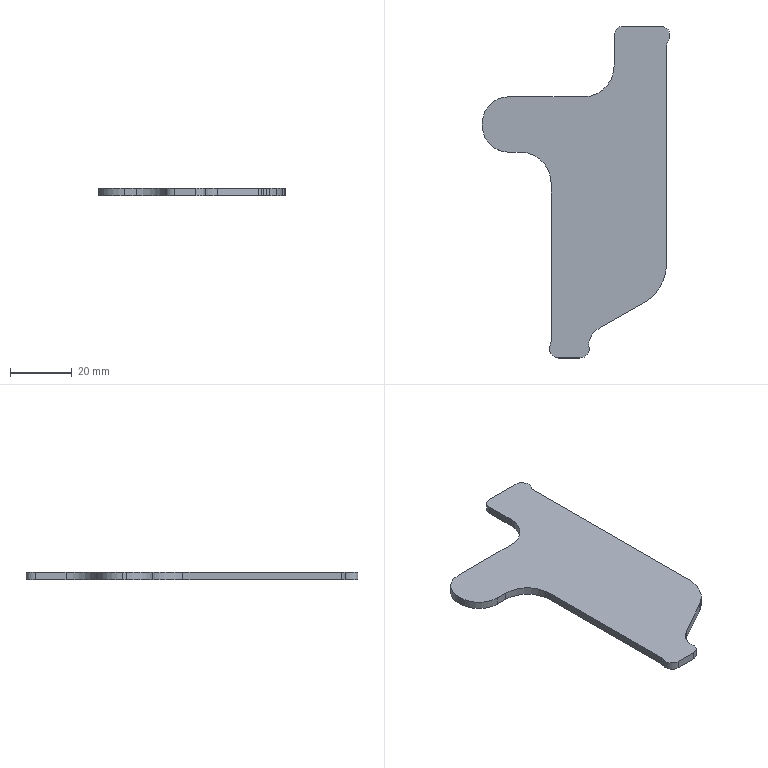Part | STEP file | lll_id354_x_t | 1 solid | 30 faces | box 60.865 x 107.859 x 2.5 mm | volume 9002 mm3 | cylinder 19 | plane 11 | commonest cylinder face diameters 6 x7 17.001 x2 20.001 x2 16.14 x1 25.107 x1 28.276 x1
STEP:
#1=CARTESIAN_POINT('',(469.5,-58.5,0.));
#2=VERTEX_POINT('',#1);
#3=CARTESIAN_POINT('',(469.5,-48.5,0.));
#4=VERTEX_POINT('',#3);
#5=CARTESIAN_POINT('',(469.5,-58.5,0.));
#6=DIRECTION('',(0.,1.,0.));
#7=VECTOR('',#6,1.);
#8=LINE('',#5,#7);
#9=EDGE_CURVE('',#2,#4,#8,.T.);
#10=ORIENTED_EDGE('',*,*,#9,.F.);
#11=CARTESIAN_POINT('',(469.5,-58.5,2.5));
#12=VERTEX_POINT('',#11);
#13=CARTESIAN_POINT('',(469.5,-58.5,2.5));
#14=DIRECTION('',(0.,0.,-1.));
#15=VECTOR('',#14,1.);
#16=LINE('',#13,#15);
#17=EDGE_CURVE('',#12,#2,#16,.T.);
#18=ORIENTED_EDGE('',*,*,#17,.F.);
#19=CARTESIAN_POINT('',(469.5,-48.5,2.5));
#20=VERTEX_POINT('',#19);
#21=CARTESIAN_POINT('',(469.5,-58.5,2.5));
#22=DIRECTION('',(0.,1.,0.));
#23=VECTOR('',#22,1.);
#24=LINE('',#21,#23);
#25=EDGE_CURVE('',#12,#20,#24,.T.);
#26=ORIENTED_EDGE('',*,*,#25,.T.);
#27=CARTESIAN_POINT('',(469.5,-48.5,-2.5));
#28=DIRECTION('',(0.,0.,1.));
#29=VECTOR('',#28,1.);
#30=LINE('',#27,#29);
#31=EDGE_CURVE('',#4,#20,#30,.T.);
#32=ORIENTED_EDGE('',*,*,#31,.F.);
#33=EDGE_LOOP('',(#10,#18,#26,#32));
#34=FACE_OUTER_BOUND('',#33,.T.);
#35=CARTESIAN_POINT('',(469.5,-58.5,2.5));
#36=DIRECTION('',(-1.,0.,0.));
#37=DIRECTION('',(0.,0.,1.));
#38=AXIS2_PLACEMENT_3D('',#35,#36,#37);
#39=PLANE('',#38);
#40=ADVANCED_FACE('',(#34),#39,.T.);
#41=CARTESIAN_POINT('',(459.5,-68.5,0.));
#42=VERTEX_POINT('',#41);
#43=CARTESIAN_POINT('',(459.499,-58.499,0.));
#44=DIRECTION('',(0.,0.,1.));
#45=DIRECTION('',(-1.,0.,0.));
#46=AXIS2_PLACEMENT_3D('',#43,#44,#45);
#47=CIRCLE('',#46,10.001);
#48=EDGE_CURVE('',#42,#2,#47,.T.);
#49=ORIENTED_EDGE('',*,*,#48,.F.);
#50=CARTESIAN_POINT('',(459.5,-68.5,2.5));
#51=VERTEX_POINT('',#50);
#52=CARTESIAN_POINT('',(459.5,-68.5,2.5));
#53=DIRECTION('',(0.,0.,-1.));
#54=VECTOR('',#53,1.);
#55=LINE('',#52,#54);
#56=EDGE_CURVE('',#51,#42,#55,.T.);
#57=ORIENTED_EDGE('',*,*,#56,.F.);
#58=CARTESIAN_POINT('',(459.499,-58.499,2.5));
#59=DIRECTION('',(0.,0.,1.));
#60=DIRECTION('',(-1.,0.,0.));
#61=AXIS2_PLACEMENT_3D('',#58,#59,#60);
#62=CIRCLE('',#61,10.001);
#63=EDGE_CURVE('',#51,#12,#62,.T.);
#64=ORIENTED_EDGE('',*,*,#63,.T.);
#65=ORIENTED_EDGE('',*,*,#17,.T.);
#66=EDGE_LOOP('',(#49,#57,#64,#65));
#67=FACE_OUTER_BOUND('',#66,.T.);
#68=CARTESIAN_POINT('',(459.499,-58.499,2.5));
#69=DIRECTION('',(0.,0.,-1.));
#70=DIRECTION('',(-1.,0.,0.));
#71=AXIS2_PLACEMENT_3D('',#68,#69,#70);
#72=CYLINDRICAL_SURFACE('',#71,10.001);
#73=ADVANCED_FACE('',(#67),#72,.F.);
#74=CARTESIAN_POINT('',(435.2,-68.5,0.));
#75=VERTEX_POINT('',#74);
#76=CARTESIAN_POINT('',(435.2,-68.5,0.));
#77=DIRECTION('',(1.,0.,0.));
#78=VECTOR('',#77,1.);
#79=LINE('',#76,#78);
#80=EDGE_CURVE('',#75,#42,#79,.T.);
#81=ORIENTED_EDGE('',*,*,#80,.F.);
#82=CARTESIAN_POINT('',(435.2,-68.5,2.5));
#83=VERTEX_POINT('',#82);
#84=CARTESIAN_POINT('',(435.2,-68.5,2.5));
#85=DIRECTION('',(0.,0.,-1.));
#86=VECTOR('',#85,1.);
#87=LINE('',#84,#86);
#88=EDGE_CURVE('',#83,#75,#87,.T.);
#89=ORIENTED_EDGE('',*,*,#88,.F.);
#90=CARTESIAN_POINT('',(435.2,-68.5,2.5));
#91=DIRECTION('',(1.,0.,0.));
#92=VECTOR('',#91,1.);
#93=LINE('',#90,#92);
#94=EDGE_CURVE('',#83,#51,#93,.T.);
#95=ORIENTED_EDGE('',*,*,#94,.T.);
#96=ORIENTED_EDGE('',*,*,#56,.T.);
#97=EDGE_LOOP('',(#81,#89,#95,#96));
#98=FACE_OUTER_BOUND('',#97,.T.);
#99=CARTESIAN_POINT('',(435.2,-68.5,2.5));
#100=DIRECTION('',(0.,1.,0.));
#101=DIRECTION('',(0.,0.,1.));
#102=AXIS2_PLACEMENT_3D('',#99,#100,#101);
#103=PLANE('',#102);
#104=ADVANCED_FACE('',(#98),#103,.T.);
#105=CARTESIAN_POINT('',(426.7,-77.,0.));
#106=VERTEX_POINT('',#105);
#107=CARTESIAN_POINT('',(435.2,-77.,0.));
#108=DIRECTION('',(0.,0.,-1.));
#109=DIRECTION('',(-1.,0.,0.));
#110=AXIS2_PLACEMENT_3D('',#107,#108,#109);
#111=CIRCLE('',#110,8.5);
#112=EDGE_CURVE('',#106,#75,#111,.T.);
#113=ORIENTED_EDGE('',*,*,#112,.F.);
#114=CARTESIAN_POINT('',(426.7,-77.,2.5));
#115=VERTEX_POINT('',#114);
#116=CARTESIAN_POINT('',(426.7,-77.,2.5));
#117=DIRECTION('',(0.,0.,-1.));
#118=VECTOR('',#117,1.);
#119=LINE('',#116,#118);
#120=EDGE_CURVE('',#115,#106,#119,.T.);
#121=ORIENTED_EDGE('',*,*,#120,.F.);
#122=CARTESIAN_POINT('',(435.2,-77.,2.5));
#123=DIRECTION('',(0.,0.,-1.));
#124=DIRECTION('',(-1.,0.,0.));
#125=AXIS2_PLACEMENT_3D('',#122,#123,#124);
#126=CIRCLE('',#125,8.5);
#127=EDGE_CURVE('',#115,#83,#126,.T.);
#128=ORIENTED_EDGE('',*,*,#127,.T.);
#129=ORIENTED_EDGE('',*,*,#88,.T.);
#130=EDGE_LOOP('',(#113,#121,#128,#129));
#131=FACE_OUTER_BOUND('',#130,.T.);
#132=CARTESIAN_POINT('',(435.2,-77.,2.5));
#133=DIRECTION('',(0.,0.,-1.));
#134=DIRECTION('',(-1.,0.,0.));
#135=AXIS2_PLACEMENT_3D('',#132,#133,#134);
#136=CYLINDRICAL_SURFACE('',#135,8.5);
#137=ADVANCED_FACE('',(#131),#136,.T.);
#138=CARTESIAN_POINT('',(426.7,-78.,0.));
#139=VERTEX_POINT('',#138);
#140=CARTESIAN_POINT('',(426.7,-78.,0.));
#141=DIRECTION('',(0.,1.,0.));
#142=VECTOR('',#141,1.);
#143=LINE('',#140,#142);
#144=EDGE_CURVE('',#139,#106,#143,.T.);
#145=ORIENTED_EDGE('',*,*,#144,.F.);
#146=CARTESIAN_POINT('',(426.7,-78.,2.5));
#147=VERTEX_POINT('',#146);
#148=CARTESIAN_POINT('',(426.7,-78.,2.5));
#149=DIRECTION('',(0.,0.,-1.));
#150=VECTOR('',#149,1.);
#151=LINE('',#148,#150);
#152=EDGE_CURVE('',#147,#139,#151,.T.);
#153=ORIENTED_EDGE('',*,*,#152,.F.);
#154=CARTESIAN_POINT('',(426.7,-78.,2.5));
#155=DIRECTION('',(0.,1.,0.));
#156=VECTOR('',#155,1.);
#157=LINE('',#154,#156);
#158=EDGE_CURVE('',#147,#115,#157,.T.);
#159=ORIENTED_EDGE('',*,*,#158,.T.);
#160=ORIENTED_EDGE('',*,*,#120,.T.);
#161=EDGE_LOOP('',(#145,#153,#159,#160));
#162=FACE_OUTER_BOUND('',#161,.T.);
#163=CARTESIAN_POINT('',(426.7,-78.,2.5));
#164=DIRECTION('',(-1.,0.,0.));
#165=DIRECTION('',(0.,0.,1.));
#166=AXIS2_PLACEMENT_3D('',#163,#164,#165);
#167=PLANE('',#166);
#168=ADVANCED_FACE('',(#162),#167,.T.);
#169=CARTESIAN_POINT('',(435.2,-86.5,0.));
#170=VERTEX_POINT('',#169);
#171=CARTESIAN_POINT('',(435.2,-78.,0.));
#172=DIRECTION('',(0.,0.,-1.));
#173=DIRECTION('',(-1.,0.,0.));
#174=AXIS2_PLACEMENT_3D('',#171,#172,#173);
#175=CIRCLE('',#174,8.5);
#176=EDGE_CURVE('',#170,#139,#175,.T.);
#177=ORIENTED_EDGE('',*,*,#176,.F.);
#178=CARTESIAN_POINT('',(435.2,-86.5,2.5));
#179=VERTEX_POINT('',#178);
#180=CARTESIAN_POINT('',(435.2,-86.5,2.5));
#181=DIRECTION('',(0.,0.,-1.));
#182=VECTOR('',#181,1.);
#183=LINE('',#180,#182);
#184=EDGE_CURVE('',#179,#170,#183,.T.);
#185=ORIENTED_EDGE('',*,*,#184,.F.);
#186=CARTESIAN_POINT('',(435.2,-78.,2.5));
#187=DIRECTION('',(0.,0.,-1.));
#188=DIRECTION('',(-1.,0.,0.));
#189=AXIS2_PLACEMENT_3D('',#186,#187,#188);
#190=CIRCLE('',#189,8.5);
#191=EDGE_CURVE('',#179,#147,#190,.T.);
#192=ORIENTED_EDGE('',*,*,#191,.T.);
#193=ORIENTED_EDGE('',*,*,#152,.T.);
#194=EDGE_LOOP('',(#177,#185,#192,#193));
#195=FACE_OUTER_BOUND('',#194,.T.);
#196=CARTESIAN_POINT('',(435.2,-78.,2.5));
#197=DIRECTION('',(0.,0.,-1.));
#198=DIRECTION('',(-1.,0.,0.));
#199=AXIS2_PLACEMENT_3D('',#196,#197,#198);
#200=CYLINDRICAL_SURFACE('',#199,8.5);
#201=ADVANCED_FACE('',(#195),#200,.T.);
#202=CARTESIAN_POINT('',(439.,-86.5,0.));
#203=VERTEX_POINT('',#202);
#204=CARTESIAN_POINT('',(439.,-86.5,0.));
#205=DIRECTION('',(-1.,0.,0.));
#206=VECTOR('',#205,1.);
#207=LINE('',#204,#206);
#208=EDGE_CURVE('',#203,#170,#207,.T.);
#209=ORIENTED_EDGE('',*,*,#208,.F.);
#210=CARTESIAN_POINT('',(439.,-86.5,2.5));
#211=VERTEX_POINT('',#210);
#212=CARTESIAN_POINT('',(439.,-86.5,2.5));
#213=DIRECTION('',(0.,0.,-1.));
#214=VECTOR('',#213,1.);
#215=LINE('',#212,#214);
#216=EDGE_CURVE('',#211,#203,#215,.T.);
#217=ORIENTED_EDGE('',*,*,#216,.F.);
#218=CARTESIAN_POINT('',(439.,-86.5,2.5));
#219=DIRECTION('',(-1.,0.,0.));
#220=VECTOR('',#219,1.);
#221=LINE('',#218,#220);
#222=EDGE_CURVE('',#211,#179,#221,.T.);
#223=ORIENTED_EDGE('',*,*,#222,.T.);
#224=ORIENTED_EDGE('',*,*,#184,.T.);
#225=EDGE_LOOP('',(#209,#217,#223,#224));
#226=FACE_OUTER_BOUND('',#225,.T.);
#227=CARTESIAN_POINT('',(439.,-86.5,2.5));
#228=DIRECTION('',(0.,-1.,0.));
#229=DIRECTION('',(0.,0.,-1.));
#230=AXIS2_PLACEMENT_3D('',#227,#228,#229);
#231=PLANE('',#230);
#232=ADVANCED_FACE('',(#226),#231,.T.);
#233=CARTESIAN_POINT('',(449.,-96.5,0.));
#234=VERTEX_POINT('',#233);
#235=CARTESIAN_POINT('',(438.999,-96.501,0.));
#236=DIRECTION('',(0.,0.,1.));
#237=DIRECTION('',(-1.,0.,0.));
#238=AXIS2_PLACEMENT_3D('',#235,#236,#237);
#239=CIRCLE('',#238,10.001);
#240=EDGE_CURVE('',#234,#203,#239,.T.);
#241=ORIENTED_EDGE('',*,*,#240,.F.);
#242=CARTESIAN_POINT('',(449.,-96.5,2.5));
#243=VERTEX_POINT('',#242);
#244=CARTESIAN_POINT('',(449.,-96.5,2.5));
#245=DIRECTION('',(0.,0.,-1.));
#246=VECTOR('',#245,1.);
#247=LINE('',#244,#246);
#248=EDGE_CURVE('',#243,#234,#247,.T.);
#249=ORIENTED_EDGE('',*,*,#248,.F.);
#250=CARTESIAN_POINT('',(438.999,-96.501,2.5));
#251=DIRECTION('',(0.,0.,1.));
#252=DIRECTION('',(-1.,0.,0.));
#253=AXIS2_PLACEMENT_3D('',#250,#251,#252);
#254=CIRCLE('',#253,10.001);
#255=EDGE_CURVE('',#243,#211,#254,.T.);
#256=ORIENTED_EDGE('',*,*,#255,.T.);
#257=ORIENTED_EDGE('',*,*,#216,.T.);
#258=EDGE_LOOP('',(#241,#249,#256,#257));
#259=FACE_OUTER_BOUND('',#258,.T.);
#260=CARTESIAN_POINT('',(438.999,-96.501,2.5));
#261=DIRECTION('',(0.,0.,-1.));
#262=DIRECTION('',(-1.,0.,0.));
#263=AXIS2_PLACEMENT_3D('',#260,#261,#262);
#264=CYLINDRICAL_SURFACE('',#263,10.001);
#265=ADVANCED_FACE('',(#259),#264,.F.);
#266=CARTESIAN_POINT('',(449.,-147.961,0.));
#267=VERTEX_POINT('',#266);
#268=CARTESIAN_POINT('',(449.,-147.961,0.));
#269=DIRECTION('',(0.,1.,0.));
#270=VECTOR('',#269,1.);
#271=LINE('',#268,#270);
#272=EDGE_CURVE('',#267,#234,#271,.T.);
#273=ORIENTED_EDGE('',*,*,#272,.F.);
#274=CARTESIAN_POINT('',(449.,-147.961,2.5));
#275=VERTEX_POINT('',#274);
#276=CARTESIAN_POINT('',(449.,-147.961,2.5));
#277=DIRECTION('',(0.,0.,-1.));
#278=VECTOR('',#277,1.);
#279=LINE('',#276,#278);
#280=EDGE_CURVE('',#275,#267,#279,.T.);
#281=ORIENTED_EDGE('',*,*,#280,.F.);
#282=CARTESIAN_POINT('',(449.,-147.961,2.5));
#283=DIRECTION('',(0.,1.,0.));
#284=VECTOR('',#283,1.);
#285=LINE('',#282,#284);
#286=EDGE_CURVE('',#275,#243,#285,.T.);
#287=ORIENTED_EDGE('',*,*,#286,.T.);
#288=ORIENTED_EDGE('',*,*,#248,.T.);
#289=EDGE_LOOP('',(#273,#281,#287,#288));
#290=FACE_OUTER_BOUND('',#289,.T.);
#291=CARTESIAN_POINT('',(449.,-147.961,2.5));
#292=DIRECTION('',(-1.,0.,0.));
#293=DIRECTION('',(0.,0.,1.));
#294=AXIS2_PLACEMENT_3D('',#291,#292,#293);
#295=PLANE('',#294);
#296=ADVANCED_FACE('',(#290),#295,.T.);
#297=CARTESIAN_POINT('',(448.75,-149.16,0.));
#298=VERTEX_POINT('',#297);
#299=CARTESIAN_POINT('',(446.,-147.961,0.));
#300=DIRECTION('',(0.,0.,1.));
#301=DIRECTION('',(-1.,0.,0.));
#302=AXIS2_PLACEMENT_3D('',#299,#300,#301);
#303=CIRCLE('',#302,3.);
#304=EDGE_CURVE('',#298,#267,#303,.T.);
#305=ORIENTED_EDGE('',*,*,#304,.F.);
#306=CARTESIAN_POINT('',(448.75,-149.16,2.5));
#307=VERTEX_POINT('',#306);
#308=CARTESIAN_POINT('',(448.75,-149.16,2.5));
#309=DIRECTION('',(0.,0.,-1.));
#310=VECTOR('',#309,1.);
#311=LINE('',#308,#310);
#312=EDGE_CURVE('',#307,#298,#311,.T.);
#313=ORIENTED_EDGE('',*,*,#312,.F.);
#314=CARTESIAN_POINT('',(446.,-147.961,2.5));
#315=DIRECTION('',(0.,0.,1.));
#316=DIRECTION('',(-1.,0.,0.));
#317=AXIS2_PLACEMENT_3D('',#314,#315,#316);
#318=CIRCLE('',#317,3.);
#319=EDGE_CURVE('',#307,#275,#318,.T.);
#320=ORIENTED_EDGE('',*,*,#319,.T.);
#321=ORIENTED_EDGE('',*,*,#280,.T.);
#322=EDGE_LOOP('',(#305,#313,#320,#321));
#323=FACE_OUTER_BOUND('',#322,.T.);
#324=CARTESIAN_POINT('',(446.,-147.961,2.5));
#325=DIRECTION('',(0.,0.,-1.));
#326=DIRECTION('',(-1.,0.,0.));
#327=AXIS2_PLACEMENT_3D('',#324,#325,#326);
#328=CYLINDRICAL_SURFACE('',#327,3.);
#329=ADVANCED_FACE('',(#323),#328,.F.);
#330=CARTESIAN_POINT('',(451.5,-153.359,0.));
#331=VERTEX_POINT('',#330);
#332=CARTESIAN_POINT('',(451.5,-150.359,0.));
#333=DIRECTION('',(0.,0.,-1.));
#334=DIRECTION('',(-1.,0.,0.));
#335=AXIS2_PLACEMENT_3D('',#332,#333,#334);
#336=CIRCLE('',#335,3.);
#337=EDGE_CURVE('',#331,#298,#336,.T.);
#338=ORIENTED_EDGE('',*,*,#337,.F.);
#339=CARTESIAN_POINT('',(451.5,-153.359,2.5));
#340=VERTEX_POINT('',#339);
#341=CARTESIAN_POINT('',(451.5,-153.359,2.5));
#342=DIRECTION('',(0.,0.,-1.));
#343=VECTOR('',#342,1.);
#344=LINE('',#341,#343);
#345=EDGE_CURVE('',#340,#331,#344,.T.);
#346=ORIENTED_EDGE('',*,*,#345,.F.);
#347=CARTESIAN_POINT('',(451.5,-150.359,2.5));
#348=DIRECTION('',(0.,0.,-1.));
#349=DIRECTION('',(-1.,0.,0.));
#350=AXIS2_PLACEMENT_3D('',#347,#348,#349);
#351=CIRCLE('',#350,3.);
#352=EDGE_CURVE('',#340,#307,#351,.T.);
#353=ORIENTED_EDGE('',*,*,#352,.T.);
#354=ORIENTED_EDGE('',*,*,#312,.T.);
#355=EDGE_LOOP('',(#338,#346,#353,#354));
#356=FACE_OUTER_BOUND('',#355,.T.);
#357=CARTESIAN_POINT('',(451.5,-150.359,2.5));
#358=DIRECTION('',(0.,0.,-1.));
#359=DIRECTION('',(-1.,0.,0.));
#360=AXIS2_PLACEMENT_3D('',#357,#358,#359);
#361=CYLINDRICAL_SURFACE('',#360,3.);
#362=ADVANCED_FACE('',(#356),#361,.T.);
#363=ORIENTED_EDGE('',*,*,#9,.T.);
#364=CARTESIAN_POINT('',(472.5,-45.5,0.));
#365=VERTEX_POINT('',#364);
#366=CARTESIAN_POINT('',(472.5,-48.5,0.));
#367=DIRECTION('',(0.,0.,-1.));
#368=DIRECTION('',(1.,0.,0.));
#369=AXIS2_PLACEMENT_3D('',#366,#367,#368);
#370=CIRCLE('',#369,3.);
#371=EDGE_CURVE('',#4,#365,#370,.T.);
#372=ORIENTED_EDGE('',*,*,#371,.T.);
#373=CARTESIAN_POINT('',(484.565,-45.5,0.));
#374=VERTEX_POINT('',#373);
#375=CARTESIAN_POINT('',(471.445,-45.5,0.));
#376=DIRECTION('',(1.,0.,0.));
#377=VECTOR('',#376,1.);
#378=LINE('',#375,#377);
#379=EDGE_CURVE('',#365,#374,#378,.T.);
#380=ORIENTED_EDGE('',*,*,#379,.T.);
#381=CARTESIAN_POINT('',(487.038,-50.199,0.));
#382=VERTEX_POINT('',#381);
#383=CARTESIAN_POINT('',(484.565,-48.5,0.));
#384=DIRECTION('',(0.,0.,-1.));
#385=DIRECTION('',(1.,0.,0.));
#386=AXIS2_PLACEMENT_3D('',#383,#384,#385);
#387=CIRCLE('',#386,3.);
#388=EDGE_CURVE('',#374,#382,#387,.T.);
#389=ORIENTED_EDGE('',*,*,#388,.T.);
#390=CARTESIAN_POINT('',(486.51,-51.898,0.));
#391=VERTEX_POINT('',#390);
#392=CARTESIAN_POINT('',(489.51,-51.898,0.));
#393=DIRECTION('',(0.,0.,-1.));
#394=DIRECTION('',(1.,0.,0.));
#395=AXIS2_PLACEMENT_3D('',#392,#393,#394);
#396=CIRCLE('',#395,3.);
#397=EDGE_CURVE('',#391,#382,#396,.T.);
#398=ORIENTED_EDGE('',*,*,#397,.F.);
#399=CARTESIAN_POINT('',(486.506,-122.731,0.));
#400=VERTEX_POINT('',#399);
#401=CARTESIAN_POINT('',(486.51,-51.898,0.));
#402=DIRECTION('',(0.00006142,1.,0.));
#403=VECTOR('',#402,1.);
#404=LINE('',#401,#403);
#405=EDGE_CURVE('',#400,#391,#404,.T.);
#406=ORIENTED_EDGE('',*,*,#405,.F.);
#407=CARTESIAN_POINT('',(486.461,-123.716,0.));
#408=VERTEX_POINT('',#407);
#409=CARTESIAN_POINT('',(439.156,-121.059,0.));
#410=DIRECTION('',(0.,0.,1.));
#411=DIRECTION('',(1.,0.,0.));
#412=AXIS2_PLACEMENT_3D('',#409,#410,#411);
#413=CIRCLE('',#412,47.38);
#414=EDGE_CURVE('',#408,#400,#413,.T.);
#415=ORIENTED_EDGE('',*,*,#414,.F.);
#416=CARTESIAN_POINT('',(484.678,-129.804,0.));
#417=VERTEX_POINT('',#416);
#418=CARTESIAN_POINT('',(472.347,-122.889,0.));
#419=DIRECTION('',(0.,0.,1.));
#420=DIRECTION('',(1.,0.,0.));
#421=AXIS2_PLACEMENT_3D('',#418,#419,#420);
#422=CIRCLE('',#421,14.138);
#423=EDGE_CURVE('',#417,#408,#422,.T.);
#424=ORIENTED_EDGE('',*,*,#423,.F.);
#425=CARTESIAN_POINT('',(482.171,-133.152,0.));
#426=VERTEX_POINT('',#425);
#427=CARTESIAN_POINT('',(472.01,-122.929,0.));
#428=DIRECTION('',(0.,0.,1.));
#429=DIRECTION('',(1.,0.,0.));
#430=AXIS2_PLACEMENT_3D('',#427,#428,#429);
#431=CIRCLE('',#430,14.414);
#432=EDGE_CURVE('',#426,#417,#431,.T.);
#433=ORIENTED_EDGE('',*,*,#432,.F.);
#434=CARTESIAN_POINT('',(481.25,-133.962,0.));
#435=VERTEX_POINT('',#434);
#436=CARTESIAN_POINT('',(473.427,-124.145,0.));
#437=DIRECTION('',(0.,0.,-1.));
#438=DIRECTION('',(1.,0.,0.));
#439=AXIS2_PLACEMENT_3D('',#436,#437,#438);
#440=CIRCLE('',#439,12.553);
#441=EDGE_CURVE('',#426,#435,#440,.T.);
#442=ORIENTED_EDGE('',*,*,#441,.T.);
#443=CARTESIAN_POINT('',(480.466,-134.556,0.));
#444=VERTEX_POINT('',#443);
#445=CARTESIAN_POINT('',(469.718,-119.534,0.));
#446=DIRECTION('',(0.,0.,1.));
#447=DIRECTION('',(1.,0.,0.));
#448=AXIS2_PLACEMENT_3D('',#445,#446,#447);
#449=CIRCLE('',#448,18.471);
#450=EDGE_CURVE('',#444,#435,#449,.T.);
#451=ORIENTED_EDGE('',*,*,#450,.F.);
#452=CARTESIAN_POINT('',(479.654,-135.117,0.));
#453=VERTEX_POINT('',#452);
#454=CARTESIAN_POINT('',(462.354,-109.242,0.));
#455=DIRECTION('',(0.,0.,-1.));
#456=DIRECTION('',(1.,0.,0.));
#457=AXIS2_PLACEMENT_3D('',#454,#455,#456);
#458=CIRCLE('',#457,31.126);
#459=EDGE_CURVE('',#444,#453,#458,.T.);
#460=ORIENTED_EDGE('',*,*,#459,.T.);
#461=CARTESIAN_POINT('',(478.829,-135.663,0.));
#462=VERTEX_POINT('',#461);
#463=CARTESIAN_POINT('',(448.181,-88.407,0.));
#464=DIRECTION('',(0.,0.,1.));
#465=DIRECTION('',(1.,0.,0.));
#466=AXIS2_PLACEMENT_3D('',#463,#464,#465);
#467=CIRCLE('',#466,56.324);
#468=EDGE_CURVE('',#462,#453,#467,.T.);
#469=ORIENTED_EDGE('',*,*,#468,.F.);
#470=CARTESIAN_POINT('',(465.269,-143.286,0.));
#471=VERTEX_POINT('',#470);
#472=CARTESIAN_POINT('',(523.122,-110.764,0.));
#473=DIRECTION('',(0.8717,0.49,0.));
#474=VECTOR('',#473,1.);
#475=LINE('',#472,#474);
#476=EDGE_CURVE('',#471,#462,#475,.T.);
#477=ORIENTED_EDGE('',*,*,#476,.F.);
#478=CARTESIAN_POINT('',(461.369,-147.727,0.));
#479=VERTEX_POINT('',#478);
#480=CARTESIAN_POINT('',(468.962,-150.461,0.));
#481=DIRECTION('',(0.,0.,-1.));
#482=DIRECTION('',(1.,0.,0.));
#483=AXIS2_PLACEMENT_3D('',#480,#481,#482);
#484=CIRCLE('',#483,8.07);
#485=EDGE_CURVE('',#479,#471,#484,.T.);
#486=ORIENTED_EDGE('',*,*,#485,.F.);
#487=CARTESIAN_POINT('',(461.302,-149.551,0.));
#488=VERTEX_POINT('',#487);
#489=CARTESIAN_POINT('',(464.191,-148.744,0.));
#490=DIRECTION('',(0.,0.,-1.));
#491=DIRECTION('',(1.,0.,0.));
#492=AXIS2_PLACEMENT_3D('',#489,#490,#491);
#493=CIRCLE('',#492,3.);
#494=EDGE_CURVE('',#488,#479,#493,.T.);
#495=ORIENTED_EDGE('',*,*,#494,.F.);
#496=CARTESIAN_POINT('',(458.413,-153.359,0.));
#497=VERTEX_POINT('',#496);
#498=CARTESIAN_POINT('',(458.413,-150.359,0.));
#499=DIRECTION('',(0.,0.,1.));
#500=DIRECTION('',(1.,0.,0.));
#501=AXIS2_PLACEMENT_3D('',#498,#499,#500);
#502=CIRCLE('',#501,3.);
#503=EDGE_CURVE('',#497,#488,#502,.T.);
#504=ORIENTED_EDGE('',*,*,#503,.F.);
#505=CARTESIAN_POINT('',(458.933,-153.359,0.));
#506=DIRECTION('',(-1.,0.,0.));
#507=VECTOR('',#506,1.);
#508=LINE('',#505,#507);
#509=EDGE_CURVE('',#497,#331,#508,.T.);
#510=ORIENTED_EDGE('',*,*,#509,.T.);
#511=ORIENTED_EDGE('',*,*,#337,.T.);
#512=ORIENTED_EDGE('',*,*,#304,.T.);
#513=ORIENTED_EDGE('',*,*,#272,.T.);
#514=ORIENTED_EDGE('',*,*,#240,.T.);
#515=ORIENTED_EDGE('',*,*,#208,.T.);
#516=ORIENTED_EDGE('',*,*,#176,.T.);
#517=ORIENTED_EDGE('',*,*,#144,.T.);
#518=ORIENTED_EDGE('',*,*,#112,.T.);
#519=ORIENTED_EDGE('',*,*,#80,.T.);
#520=ORIENTED_EDGE('',*,*,#48,.T.);
#521=EDGE_LOOP('',(#363,#372,#380,#389,#398,#406,#415,#424,#433,#442,#451,#460,#469,#477,#486,#495,#504,#510,#511,#512,#513,#514,#515,#516,#517,#518,#519,#520));
#522=FACE_OUTER_BOUND('',#521,.T.);
#523=CARTESIAN_POINT('',(490.03,-51.898,0.));
#524=DIRECTION('',(0.,0.,1.));
#525=DIRECTION('',(1.,0.,0.));
#526=AXIS2_PLACEMENT_3D('',#523,#524,#525);
#527=PLANE('',#526);
#528=ADVANCED_FACE('',(#522),#527,.F.);
#529=CARTESIAN_POINT('',(472.5,-45.5,2.5));
#530=VERTEX_POINT('',#529);
#531=CARTESIAN_POINT('',(472.5,-48.5,2.5));
#532=DIRECTION('',(0.,0.,-1.));
#533=DIRECTION('',(1.,0.,0.));
#534=AXIS2_PLACEMENT_3D('',#531,#532,#533);
#535=CIRCLE('',#534,3.);
#536=EDGE_CURVE('',#20,#530,#535,.T.);
#537=ORIENTED_EDGE('',*,*,#536,.F.);
#538=ORIENTED_EDGE('',*,*,#25,.F.);
#539=ORIENTED_EDGE('',*,*,#63,.F.);
#540=ORIENTED_EDGE('',*,*,#94,.F.);
#541=ORIENTED_EDGE('',*,*,#127,.F.);
#542=ORIENTED_EDGE('',*,*,#158,.F.);
#543=ORIENTED_EDGE('',*,*,#191,.F.);
#544=ORIENTED_EDGE('',*,*,#222,.F.);
#545=ORIENTED_EDGE('',*,*,#255,.F.);
#546=ORIENTED_EDGE('',*,*,#286,.F.);
#547=ORIENTED_EDGE('',*,*,#319,.F.);
#548=ORIENTED_EDGE('',*,*,#352,.F.);
#549=CARTESIAN_POINT('',(458.413,-153.359,2.5));
#550=VERTEX_POINT('',#549);
#551=CARTESIAN_POINT('',(458.933,-153.359,2.5));
#552=DIRECTION('',(-1.,0.,0.));
#553=VECTOR('',#552,1.);
#554=LINE('',#551,#553);
#555=EDGE_CURVE('',#550,#340,#554,.T.);
#556=ORIENTED_EDGE('',*,*,#555,.F.);
#557=CARTESIAN_POINT('',(461.302,-149.551,2.5));
#558=VERTEX_POINT('',#557);
#559=CARTESIAN_POINT('',(458.413,-150.359,2.5));
#560=DIRECTION('',(0.,0.,-1.));
#561=DIRECTION('',(1.,0.,0.));
#562=AXIS2_PLACEMENT_3D('',#559,#560,#561);
#563=CIRCLE('',#562,3.);
#564=EDGE_CURVE('',#558,#550,#563,.T.);
#565=ORIENTED_EDGE('',*,*,#564,.F.);
#566=CARTESIAN_POINT('',(461.369,-147.727,2.5));
#567=VERTEX_POINT('',#566);
#568=CARTESIAN_POINT('',(464.191,-148.744,2.5));
#569=DIRECTION('',(0.,0.,1.));
#570=DIRECTION('',(1.,0.,0.));
#571=AXIS2_PLACEMENT_3D('',#568,#569,#570);
#572=CIRCLE('',#571,3.);
#573=EDGE_CURVE('',#567,#558,#572,.T.);
#574=ORIENTED_EDGE('',*,*,#573,.F.);
#575=CARTESIAN_POINT('',(465.269,-143.286,2.5));
#576=VERTEX_POINT('',#575);
#577=CARTESIAN_POINT('',(468.962,-150.461,2.5));
#578=DIRECTION('',(0.,0.,1.));
#579=DIRECTION('',(1.,0.,0.));
#580=AXIS2_PLACEMENT_3D('',#577,#578,#579);
#581=CIRCLE('',#580,8.07);
#582=EDGE_CURVE('',#576,#567,#581,.T.);
#583=ORIENTED_EDGE('',*,*,#582,.F.);
#584=CARTESIAN_POINT('',(478.829,-135.663,2.5));
#585=VERTEX_POINT('',#584);
#586=CARTESIAN_POINT('',(523.122,-110.764,2.5));
#587=DIRECTION('',(-0.8717,-0.49,0.));
#588=VECTOR('',#587,1.);
#589=LINE('',#586,#588);
#590=EDGE_CURVE('',#585,#576,#589,.T.);
#591=ORIENTED_EDGE('',*,*,#590,.F.);
#592=CARTESIAN_POINT('',(479.654,-135.117,2.5));
#593=VERTEX_POINT('',#592);
#594=CARTESIAN_POINT('',(448.181,-88.407,2.5));
#595=DIRECTION('',(0.,0.,1.));
#596=DIRECTION('',(1.,0.,0.));
#597=AXIS2_PLACEMENT_3D('',#594,#595,#596);
#598=CIRCLE('',#597,56.324);
#599=EDGE_CURVE('',#585,#593,#598,.T.);
#600=ORIENTED_EDGE('',*,*,#599,.T.);
#601=CARTESIAN_POINT('',(480.466,-134.556,2.5));
#602=VERTEX_POINT('',#601);
#603=CARTESIAN_POINT('',(462.354,-109.242,2.5));
#604=DIRECTION('',(0.,0.,1.));
#605=DIRECTION('',(1.,0.,0.));
#606=AXIS2_PLACEMENT_3D('',#603,#604,#605);
#607=CIRCLE('',#606,31.126);
#608=EDGE_CURVE('',#593,#602,#607,.T.);
#609=ORIENTED_EDGE('',*,*,#608,.T.);
#610=CARTESIAN_POINT('',(481.25,-133.962,2.5));
#611=VERTEX_POINT('',#610);
#612=CARTESIAN_POINT('',(469.718,-119.534,2.5));
#613=DIRECTION('',(0.,0.,1.));
#614=DIRECTION('',(1.,0.,0.));
#615=AXIS2_PLACEMENT_3D('',#612,#613,#614);
#616=CIRCLE('',#615,18.471);
#617=EDGE_CURVE('',#602,#611,#616,.T.);
#618=ORIENTED_EDGE('',*,*,#617,.T.);
#619=CARTESIAN_POINT('',(482.171,-133.152,2.5));
#620=VERTEX_POINT('',#619);
#621=CARTESIAN_POINT('',(473.427,-124.145,2.5));
#622=DIRECTION('',(0.,0.,-1.));
#623=DIRECTION('',(1.,0.,0.));
#624=AXIS2_PLACEMENT_3D('',#621,#622,#623);
#625=CIRCLE('',#624,12.553);
#626=EDGE_CURVE('',#620,#611,#625,.T.);
#627=ORIENTED_EDGE('',*,*,#626,.F.);
#628=CARTESIAN_POINT('',(484.678,-129.804,2.5));
#629=VERTEX_POINT('',#628);
#630=CARTESIAN_POINT('',(472.01,-122.929,2.5));
#631=DIRECTION('',(0.,0.,-1.));
#632=DIRECTION('',(1.,0.,0.));
#633=AXIS2_PLACEMENT_3D('',#630,#631,#632);
#634=CIRCLE('',#633,14.414);
#635=EDGE_CURVE('',#629,#620,#634,.T.);
#636=ORIENTED_EDGE('',*,*,#635,.F.);
#637=CARTESIAN_POINT('',(486.461,-123.716,2.5));
#638=VERTEX_POINT('',#637);
#639=CARTESIAN_POINT('',(472.347,-122.889,2.5));
#640=DIRECTION('',(0.,0.,-1.));
#641=DIRECTION('',(1.,0.,0.));
#642=AXIS2_PLACEMENT_3D('',#639,#640,#641);
#643=CIRCLE('',#642,14.138);
#644=EDGE_CURVE('',#638,#629,#643,.T.);
#645=ORIENTED_EDGE('',*,*,#644,.F.);
#646=CARTESIAN_POINT('',(486.506,-122.731,2.5));
#647=VERTEX_POINT('',#646);
#648=CARTESIAN_POINT('',(439.156,-121.059,2.5));
#649=DIRECTION('',(0.,0.,-1.));
#650=DIRECTION('',(1.,0.,0.));
#651=AXIS2_PLACEMENT_3D('',#648,#649,#650);
#652=CIRCLE('',#651,47.38);
#653=EDGE_CURVE('',#647,#638,#652,.T.);
#654=ORIENTED_EDGE('',*,*,#653,.F.);
#655=CARTESIAN_POINT('',(486.51,-51.898,2.5));
#656=VERTEX_POINT('',#655);
#657=CARTESIAN_POINT('',(486.51,-51.898,2.5));
#658=DIRECTION('',(0.00006142,1.,0.));
#659=VECTOR('',#658,1.);
#660=LINE('',#657,#659);
#661=EDGE_CURVE('',#647,#656,#660,.T.);
#662=ORIENTED_EDGE('',*,*,#661,.T.);
#663=CARTESIAN_POINT('',(487.038,-50.199,2.5));
#664=VERTEX_POINT('',#663);
#665=CARTESIAN_POINT('',(489.51,-51.898,2.5));
#666=DIRECTION('',(0.,0.,-1.));
#667=DIRECTION('',(1.,0.,0.));
#668=AXIS2_PLACEMENT_3D('',#665,#666,#667);
#669=CIRCLE('',#668,3.);
#670=EDGE_CURVE('',#656,#664,#669,.T.);
#671=ORIENTED_EDGE('',*,*,#670,.T.);
#672=CARTESIAN_POINT('',(484.565,-45.5,2.5));
#673=VERTEX_POINT('',#672);
#674=CARTESIAN_POINT('',(484.565,-48.5,2.5));
#675=DIRECTION('',(0.,0.,-1.));
#676=DIRECTION('',(1.,0.,0.));
#677=AXIS2_PLACEMENT_3D('',#674,#675,#676);
#678=CIRCLE('',#677,3.);
#679=EDGE_CURVE('',#673,#664,#678,.T.);
#680=ORIENTED_EDGE('',*,*,#679,.F.);
#681=CARTESIAN_POINT('',(471.445,-45.5,2.5));
#682=DIRECTION('',(1.,0.,0.));
#683=VECTOR('',#682,1.);
#684=LINE('',#681,#683);
#685=EDGE_CURVE('',#530,#673,#684,.T.);
#686=ORIENTED_EDGE('',*,*,#685,.F.);
#687=EDGE_LOOP('',(#537,#538,#539,#540,#541,#542,#543,#544,#545,#546,#547,#548,#556,#565,#574,#583,#591,#600,#609,#618,#627,#636,#645,#654,#662,#671,#680,#686));
#688=FACE_OUTER_BOUND('',#687,.T.);
#689=CARTESIAN_POINT('',(490.03,-51.898,2.5));
#690=DIRECTION('',(0.,0.,1.));
#691=DIRECTION('',(1.,0.,0.));
#692=AXIS2_PLACEMENT_3D('',#689,#690,#691);
#693=PLANE('',#692);
#694=ADVANCED_FACE('',(#688),#693,.T.);
#695=CARTESIAN_POINT('',(472.5,-45.5,-2.5));
#696=DIRECTION('',(0.,0.,-1.));
#697=VECTOR('',#696,1.);
#698=LINE('',#695,#697);
#699=EDGE_CURVE('',#530,#365,#698,.T.);
#700=ORIENTED_EDGE('',*,*,#699,.F.);
#701=ORIENTED_EDGE('',*,*,#685,.T.);
#702=CARTESIAN_POINT('',(484.565,-45.5,-2.5));
#703=DIRECTION('',(0.,0.,1.));
#704=VECTOR('',#703,1.);
#705=LINE('',#702,#704);
#706=EDGE_CURVE('',#374,#673,#705,.T.);
#707=ORIENTED_EDGE('',*,*,#706,.F.);
#708=ORIENTED_EDGE('',*,*,#379,.F.);
#709=EDGE_LOOP('',(#700,#701,#707,#708));
#710=FACE_OUTER_BOUND('',#709,.T.);
#711=CARTESIAN_POINT('',(471.445,-45.5,2.5));
#712=DIRECTION('',(0.,1.,0.));
#713=DIRECTION('',(1.,0.,0.));
#714=AXIS2_PLACEMENT_3D('',#711,#712,#713);
#715=PLANE('',#714);
#716=ADVANCED_FACE('',(#710),#715,.T.);
#717=CARTESIAN_POINT('',(458.413,-153.359,-2.5));
#718=DIRECTION('',(0.,0.,-1.));
#719=VECTOR('',#718,1.);
#720=LINE('',#717,#719);
#721=EDGE_CURVE('',#550,#497,#720,.T.);
#722=ORIENTED_EDGE('',*,*,#721,.F.);
#723=ORIENTED_EDGE('',*,*,#555,.T.);
#724=ORIENTED_EDGE('',*,*,#345,.T.);
#725=ORIENTED_EDGE('',*,*,#509,.F.);
#726=EDGE_LOOP('',(#722,#723,#724,#725));
#727=FACE_OUTER_BOUND('',#726,.T.);
#728=CARTESIAN_POINT('',(458.933,-153.359,2.5));
#729=DIRECTION('',(0.,-1.,0.));
#730=DIRECTION('',(0.,0.,-1.));
#731=AXIS2_PLACEMENT_3D('',#728,#729,#730);
#732=PLANE('',#731);
#733=ADVANCED_FACE('',(#727),#732,.T.);
#734=ORIENTED_EDGE('',*,*,#679,.T.);
#735=CARTESIAN_POINT('',(487.038,-50.199,-2.5));
#736=DIRECTION('',(0.,0.,-1.));
#737=VECTOR('',#736,1.);
#738=LINE('',#735,#737);
#739=EDGE_CURVE('',#664,#382,#738,.T.);
#740=ORIENTED_EDGE('',*,*,#739,.T.);
#741=ORIENTED_EDGE('',*,*,#388,.F.);
#742=ORIENTED_EDGE('',*,*,#706,.T.);
#743=EDGE_LOOP('',(#734,#740,#741,#742));
#744=FACE_OUTER_BOUND('',#743,.T.);
#745=CARTESIAN_POINT('',(484.565,-48.5,-2.5));
#746=DIRECTION('',(0.,0.,1.));
#747=DIRECTION('',(1.,0.,0.));
#748=AXIS2_PLACEMENT_3D('',#745,#746,#747);
#749=CYLINDRICAL_SURFACE('',#748,3.);
#750=ADVANCED_FACE('',(#744),#749,.T.);
#751=ORIENTED_EDGE('',*,*,#670,.F.);
#752=CARTESIAN_POINT('',(486.51,-51.898,-2.5));
#753=DIRECTION('',(0.,0.,-1.));
#754=VECTOR('',#753,1.);
#755=LINE('',#752,#754);
#756=EDGE_CURVE('',#656,#391,#755,.T.);
#757=ORIENTED_EDGE('',*,*,#756,.T.);
#758=ORIENTED_EDGE('',*,*,#397,.T.);
#759=ORIENTED_EDGE('',*,*,#739,.F.);
#760=EDGE_LOOP('',(#751,#757,#758,#759));
#761=FACE_OUTER_BOUND('',#760,.T.);
#762=CARTESIAN_POINT('',(489.51,-51.898,-2.5));
#763=DIRECTION('',(0.,0.,1.));
#764=DIRECTION('',(1.,0.,0.));
#765=AXIS2_PLACEMENT_3D('',#762,#763,#764);
#766=CYLINDRICAL_SURFACE('',#765,3.);
#767=ADVANCED_FACE('',(#761),#766,.F.);
#768=ORIENTED_EDGE('',*,*,#661,.F.);
#769=CARTESIAN_POINT('',(486.506,-122.731,-2.5));
#770=DIRECTION('',(0.,0.,-1.));
#771=VECTOR('',#770,1.);
#772=LINE('',#769,#771);
#773=EDGE_CURVE('',#647,#400,#772,.T.);
#774=ORIENTED_EDGE('',*,*,#773,.T.);
#775=ORIENTED_EDGE('',*,*,#405,.T.);
#776=ORIENTED_EDGE('',*,*,#756,.F.);
#777=EDGE_LOOP('',(#768,#774,#775,#776));
#778=FACE_OUTER_BOUND('',#777,.T.);
#779=CARTESIAN_POINT('',(486.51,-51.898,-2.5));
#780=DIRECTION('',(-1.,0.00006142,0.));
#781=DIRECTION('',(-0.00006142,-1.,0.));
#782=AXIS2_PLACEMENT_3D('',#779,#780,#781);
#783=PLANE('',#782);
#784=ADVANCED_FACE('',(#778),#783,.F.);
#785=ORIENTED_EDGE('',*,*,#653,.T.);
#786=CARTESIAN_POINT('',(486.461,-123.716,-2.5));
#787=DIRECTION('',(0.,0.,-1.));
#788=VECTOR('',#787,1.);
#789=LINE('',#786,#788);
#790=EDGE_CURVE('',#638,#408,#789,.T.);
#791=ORIENTED_EDGE('',*,*,#790,.T.);
#792=ORIENTED_EDGE('',*,*,#414,.T.);
#793=ORIENTED_EDGE('',*,*,#773,.F.);
#794=EDGE_LOOP('',(#785,#791,#792,#793));
#795=FACE_OUTER_BOUND('',#794,.T.);
#796=CARTESIAN_POINT('',(439.156,-121.059,-2.5));
#797=DIRECTION('',(0.,0.,1.));
#798=DIRECTION('',(1.,0.,0.));
#799=AXIS2_PLACEMENT_3D('',#796,#797,#798);
#800=CYLINDRICAL_SURFACE('',#799,47.38);
#801=ADVANCED_FACE('',(#795),#800,.T.);
#802=ORIENTED_EDGE('',*,*,#644,.T.);
#803=CARTESIAN_POINT('',(484.678,-129.804,-2.5));
#804=DIRECTION('',(0.,0.,-1.));
#805=VECTOR('',#804,1.);
#806=LINE('',#803,#805);
#807=EDGE_CURVE('',#629,#417,#806,.T.);
#808=ORIENTED_EDGE('',*,*,#807,.T.);
#809=ORIENTED_EDGE('',*,*,#423,.T.);
#810=ORIENTED_EDGE('',*,*,#790,.F.);
#811=EDGE_LOOP('',(#802,#808,#809,#810));
#812=FACE_OUTER_BOUND('',#811,.T.);
#813=CARTESIAN_POINT('',(472.347,-122.889,-2.5));
#814=DIRECTION('',(0.,0.,1.));
#815=DIRECTION('',(1.,0.,0.));
#816=AXIS2_PLACEMENT_3D('',#813,#814,#815);
#817=CYLINDRICAL_SURFACE('',#816,14.138);
#818=ADVANCED_FACE('',(#812),#817,.T.);
#819=ORIENTED_EDGE('',*,*,#635,.T.);
#820=CARTESIAN_POINT('',(482.171,-133.152,-2.5));
#821=DIRECTION('',(0.,0.,-1.));
#822=VECTOR('',#821,1.);
#823=LINE('',#820,#822);
#824=EDGE_CURVE('',#620,#426,#823,.T.);
#825=ORIENTED_EDGE('',*,*,#824,.T.);
#826=ORIENTED_EDGE('',*,*,#432,.T.);
#827=ORIENTED_EDGE('',*,*,#807,.F.);
#828=EDGE_LOOP('',(#819,#825,#826,#827));
#829=FACE_OUTER_BOUND('',#828,.T.);
#830=CARTESIAN_POINT('',(472.01,-122.929,-2.5));
#831=DIRECTION('',(0.,0.,1.));
#832=DIRECTION('',(1.,0.,0.));
#833=AXIS2_PLACEMENT_3D('',#830,#831,#832);
#834=CYLINDRICAL_SURFACE('',#833,14.414);
#835=ADVANCED_FACE('',(#829),#834,.T.);
#836=ORIENTED_EDGE('',*,*,#626,.T.);
#837=CARTESIAN_POINT('',(481.25,-133.962,-2.5));
#838=DIRECTION('',(0.,0.,-1.));
#839=VECTOR('',#838,1.);
#840=LINE('',#837,#839);
#841=EDGE_CURVE('',#611,#435,#840,.T.);
#842=ORIENTED_EDGE('',*,*,#841,.T.);
#843=ORIENTED_EDGE('',*,*,#441,.F.);
#844=ORIENTED_EDGE('',*,*,#824,.F.);
#845=EDGE_LOOP('',(#836,#842,#843,#844));
#846=FACE_OUTER_BOUND('',#845,.T.);
#847=CARTESIAN_POINT('',(473.427,-124.145,-2.5));
#848=DIRECTION('',(0.,0.,1.));
#849=DIRECTION('',(1.,0.,0.));
#850=AXIS2_PLACEMENT_3D('',#847,#848,#849);
#851=CYLINDRICAL_SURFACE('',#850,12.553);
#852=ADVANCED_FACE('',(#846),#851,.T.);
#853=ORIENTED_EDGE('',*,*,#617,.F.);
#854=CARTESIAN_POINT('',(480.466,-134.556,-2.5));
#855=DIRECTION('',(0.,0.,-1.));
#856=VECTOR('',#855,1.);
#857=LINE('',#854,#856);
#858=EDGE_CURVE('',#602,#444,#857,.T.);
#859=ORIENTED_EDGE('',*,*,#858,.T.);
#860=ORIENTED_EDGE('',*,*,#450,.T.);
#861=ORIENTED_EDGE('',*,*,#841,.F.);
#862=EDGE_LOOP('',(#853,#859,#860,#861));
#863=FACE_OUTER_BOUND('',#862,.T.);
#864=CARTESIAN_POINT('',(469.718,-119.534,-2.5));
#865=DIRECTION('',(0.,0.,1.));
#866=DIRECTION('',(1.,0.,0.));
#867=AXIS2_PLACEMENT_3D('',#864,#865,#866);
#868=CYLINDRICAL_SURFACE('',#867,18.471);
#869=ADVANCED_FACE('',(#863),#868,.T.);
#870=ORIENTED_EDGE('',*,*,#608,.F.);
#871=CARTESIAN_POINT('',(479.654,-135.117,-2.5));
#872=DIRECTION('',(0.,0.,-1.));
#873=VECTOR('',#872,1.);
#874=LINE('',#871,#873);
#875=EDGE_CURVE('',#593,#453,#874,.T.);
#876=ORIENTED_EDGE('',*,*,#875,.T.);
#877=ORIENTED_EDGE('',*,*,#459,.F.);
#878=ORIENTED_EDGE('',*,*,#858,.F.);
#879=EDGE_LOOP('',(#870,#876,#877,#878));
#880=FACE_OUTER_BOUND('',#879,.T.);
#881=CARTESIAN_POINT('',(462.354,-109.242,-2.5));
#882=DIRECTION('',(0.,0.,1.));
#883=DIRECTION('',(1.,0.,0.));
#884=AXIS2_PLACEMENT_3D('',#881,#882,#883);
#885=CYLINDRICAL_SURFACE('',#884,31.126);
#886=ADVANCED_FACE('',(#880),#885,.T.);
#887=ORIENTED_EDGE('',*,*,#599,.F.);
#888=CARTESIAN_POINT('',(478.829,-135.663,-2.5));
#889=DIRECTION('',(0.,0.,-1.));
#890=VECTOR('',#889,1.);
#891=LINE('',#888,#890);
#892=EDGE_CURVE('',#585,#462,#891,.T.);
#893=ORIENTED_EDGE('',*,*,#892,.T.);
#894=ORIENTED_EDGE('',*,*,#468,.T.);
#895=ORIENTED_EDGE('',*,*,#875,.F.);
#896=EDGE_LOOP('',(#887,#893,#894,#895));
#897=FACE_OUTER_BOUND('',#896,.T.);
#898=CARTESIAN_POINT('',(448.181,-88.407,-2.5));
#899=DIRECTION('',(0.,0.,1.));
#900=DIRECTION('',(1.,0.,0.));
#901=AXIS2_PLACEMENT_3D('',#898,#899,#900);
#902=CYLINDRICAL_SURFACE('',#901,56.324);
#903=ADVANCED_FACE('',(#897),#902,.T.);
#904=ORIENTED_EDGE('',*,*,#590,.T.);
#905=CARTESIAN_POINT('',(465.269,-143.286,-2.5));
#906=DIRECTION('',(0.,0.,-1.));
#907=VECTOR('',#906,1.);
#908=LINE('',#905,#907);
#909=EDGE_CURVE('',#576,#471,#908,.T.);
#910=ORIENTED_EDGE('',*,*,#909,.T.);
#911=ORIENTED_EDGE('',*,*,#476,.T.);
#912=ORIENTED_EDGE('',*,*,#892,.F.);
#913=EDGE_LOOP('',(#904,#910,#911,#912));
#914=FACE_OUTER_BOUND('',#913,.T.);
#915=CARTESIAN_POINT('',(478.829,-135.663,-2.5));
#916=DIRECTION('',(-0.49,0.8717,0.));
#917=DIRECTION('',(-0.8717,-0.49,0.));
#918=AXIS2_PLACEMENT_3D('',#915,#916,#917);
#919=PLANE('',#918);
#920=ADVANCED_FACE('',(#914),#919,.F.);
#921=ORIENTED_EDGE('',*,*,#582,.T.);
#922=CARTESIAN_POINT('',(461.369,-147.727,-2.5));
#923=DIRECTION('',(0.,0.,-1.));
#924=VECTOR('',#923,1.);
#925=LINE('',#922,#924);
#926=EDGE_CURVE('',#567,#479,#925,.T.);
#927=ORIENTED_EDGE('',*,*,#926,.T.);
#928=ORIENTED_EDGE('',*,*,#485,.T.);
#929=ORIENTED_EDGE('',*,*,#909,.F.);
#930=EDGE_LOOP('',(#921,#927,#928,#929));
#931=FACE_OUTER_BOUND('',#930,.T.);
#932=CARTESIAN_POINT('',(468.962,-150.461,-2.5));
#933=DIRECTION('',(0.,0.,1.));
#934=DIRECTION('',(1.,0.,0.));
#935=AXIS2_PLACEMENT_3D('',#932,#933,#934);
#936=CYLINDRICAL_SURFACE('',#935,8.07);
#937=ADVANCED_FACE('',(#931),#936,.F.);
#938=ORIENTED_EDGE('',*,*,#573,.T.);
#939=CARTESIAN_POINT('',(461.302,-149.551,-2.5));
#940=DIRECTION('',(0.,0.,-1.));
#941=VECTOR('',#940,1.);
#942=LINE('',#939,#941);
#943=EDGE_CURVE('',#558,#488,#942,.T.);
#944=ORIENTED_EDGE('',*,*,#943,.T.);
#945=ORIENTED_EDGE('',*,*,#494,.T.);
#946=ORIENTED_EDGE('',*,*,#926,.F.);
#947=EDGE_LOOP('',(#938,#944,#945,#946));
#948=FACE_OUTER_BOUND('',#947,.T.);
#949=CARTESIAN_POINT('',(464.191,-148.744,-2.5));
#950=DIRECTION('',(0.,0.,1.));
#951=DIRECTION('',(1.,0.,0.));
#952=AXIS2_PLACEMENT_3D('',#949,#950,#951);
#953=CYLINDRICAL_SURFACE('',#952,3.);
#954=ADVANCED_FACE('',(#948),#953,.F.);
#955=ORIENTED_EDGE('',*,*,#564,.T.);
#956=ORIENTED_EDGE('',*,*,#721,.T.);
#957=ORIENTED_EDGE('',*,*,#503,.T.);
#958=ORIENTED_EDGE('',*,*,#943,.F.);
#959=EDGE_LOOP('',(#955,#956,#957,#958));
#960=FACE_OUTER_BOUND('',#959,.T.);
#961=CARTESIAN_POINT('',(458.413,-150.359,-2.5));
#962=DIRECTION('',(0.,0.,1.));
#963=DIRECTION('',(1.,0.,0.));
#964=AXIS2_PLACEMENT_3D('',#961,#962,#963);
#965=CYLINDRICAL_SURFACE('',#964,3.);
#966=ADVANCED_FACE('',(#960),#965,.T.);
#967=ORIENTED_EDGE('',*,*,#31,.T.);
#968=ORIENTED_EDGE('',*,*,#536,.T.);
#969=ORIENTED_EDGE('',*,*,#699,.T.);
#970=ORIENTED_EDGE('',*,*,#371,.F.);
#971=EDGE_LOOP('',(#967,#968,#969,#970));
#972=FACE_OUTER_BOUND('',#971,.T.);
#973=CARTESIAN_POINT('',(472.5,-48.5,-2.5));
#974=DIRECTION('',(0.,0.,1.));
#975=DIRECTION('',(1.,0.,0.));
#976=AXIS2_PLACEMENT_3D('',#973,#974,#975);
#977=CYLINDRICAL_SURFACE('',#976,3.);
#978=ADVANCED_FACE('',(#972),#977,.T.);
#979=CLOSED_SHELL('',(#40,#73,#104,#137,#168,#201,#232,#265,#296,#329,#362,#528,#694,#716,#733,#750,#767,#784,#801,#818,#835,#852,#869,#886,#903,#920,#937,#954,#966,#978));
#980=MANIFOLD_SOLID_BREP('',#979);
#981=(LENGTH_UNIT()NAMED_UNIT(*)SI_UNIT(.MILLI.,.METRE.));
#982=UNCERTAINTY_MEASURE_WITH_UNIT(LENGTH_MEASURE(0.00002),#981,'','');
#983=(NAMED_UNIT(*)PLANE_ANGLE_UNIT()SI_UNIT($,.RADIAN.));
#984=PLANE_ANGLE_MEASURE_WITH_UNIT(PLANE_ANGLE_MEASURE(0.01745),#983);
#985=DIMENSIONAL_EXPONENTS(0.,0.,0.,0.,0.,0.,0.);
#986=(CONVERSION_BASED_UNIT('DEGREE',#984)NAMED_UNIT(#985)PLANE_ANGLE_UNIT());
#987=(NAMED_UNIT(*)SI_UNIT($,.STERADIAN.)SOLID_ANGLE_UNIT());
#988=(GEOMETRIC_REPRESENTATION_CONTEXT(3)GLOBAL_UNCERTAINTY_ASSIGNED_CONTEXT((#982))GLOBAL_UNIT_ASSIGNED_CONTEXT((#981,#986,#987))REPRESENTATION_CONTEXT('',''));
#989=ADVANCED_BREP_SHAPE_REPRESENTATION('',(#980),#988);